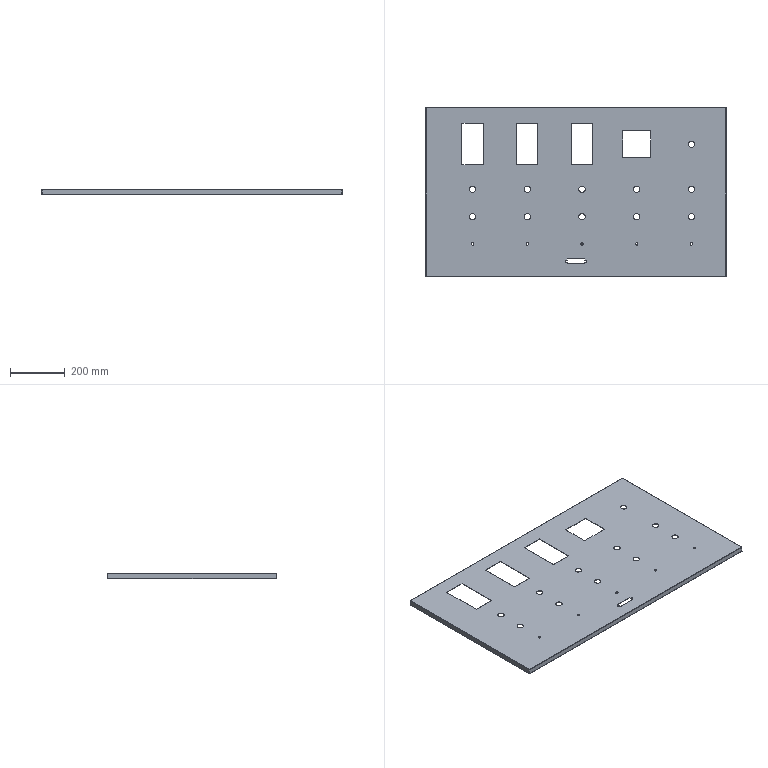Part | SolidWorks | features EdgeFlange 2, ICE 2, FlatPattern 1, SMBaseFlange 1, SheetMetal 1 | 1 solid | 131 faces | box 1100 x 620 x 20 mm | volume 1080338 mm3 | plane 64 | cylinder 51 | spline 16 | commonest cylinder face diameters 23 x22 9 x10 0.2 x8 3.2 x8 7 x3